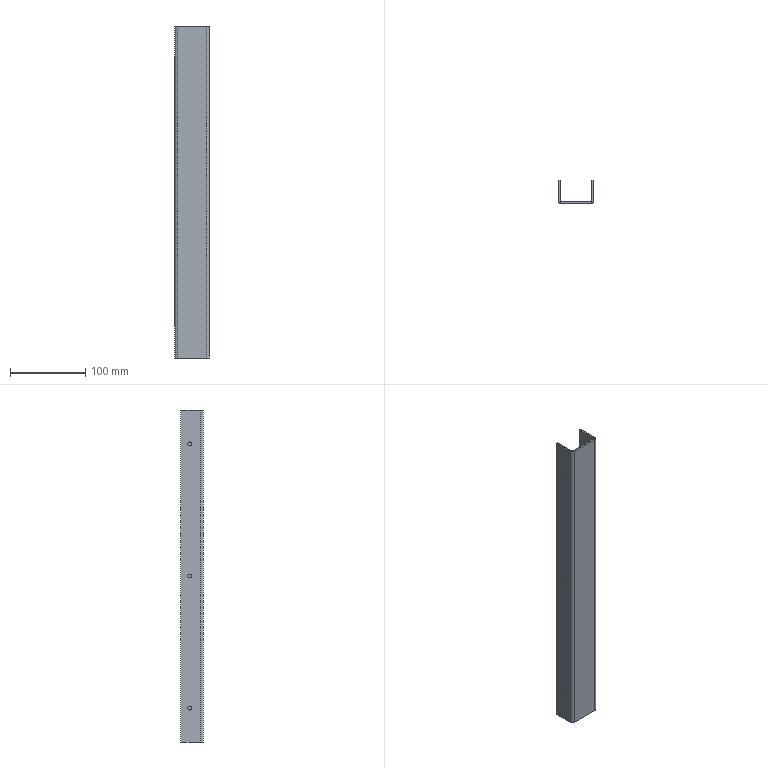Part | STEP file | 1 solid | 44 faces | box 46 x 30 x 440 mm | volume 87123 mm3 | cylinder 26 | plane 18 | commonest cylinder face diameters 7 x18 5.3 x6 3 x2